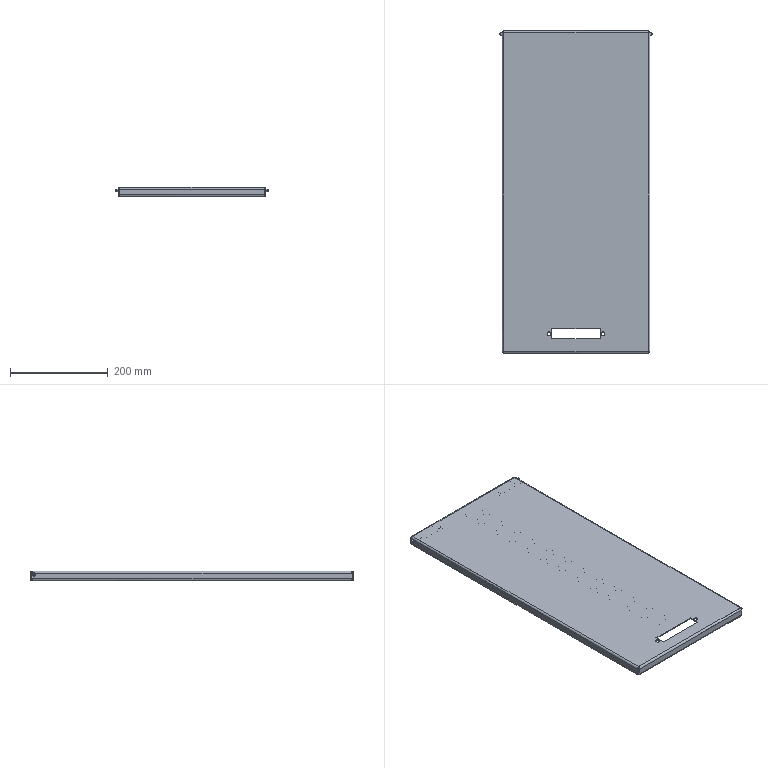Part | NX | features BREP 8 | 8 solids | 268 faces | box 312 x 659 x 20 mm | volume 566468 mm3 | plane 104 | torus 76 | cylinder 68 | spline 16 | cone 4 | commonest cylinder face diameters 6 x16 4 x12 8 x12 10 x12 5.3 x8 7 x8